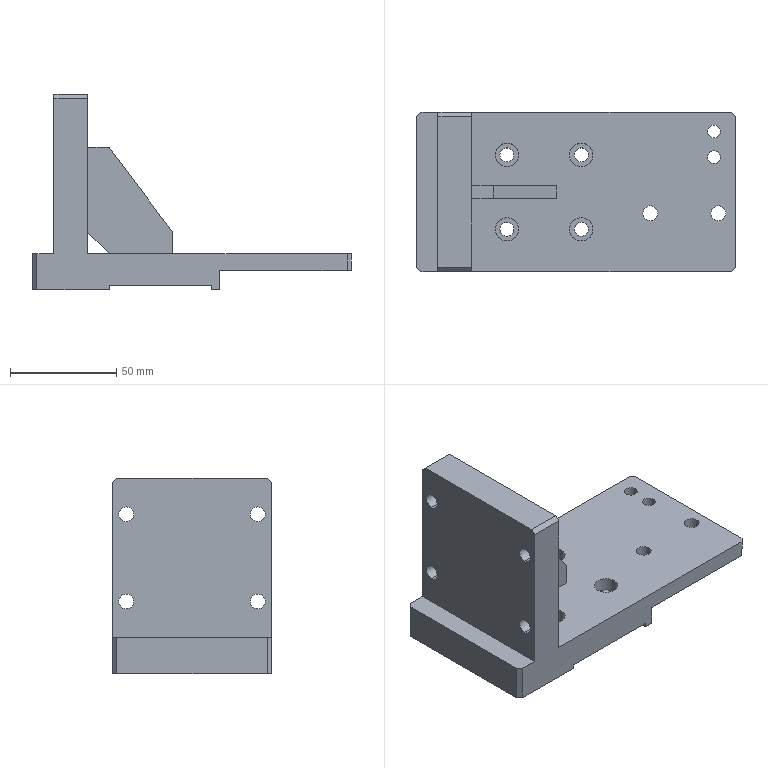Part | SolidWorks | features HoleWzd 4, ICE 4, Chamfer 1, Extrusion 1 | 1 solid | 64 faces | box 150 x 75 x 92 mm | volume 232995 mm3 | cylinder 32 | plane 32 | commonest cylinder face diameters 7 x12 6.6 x8 11 x8 6 x4